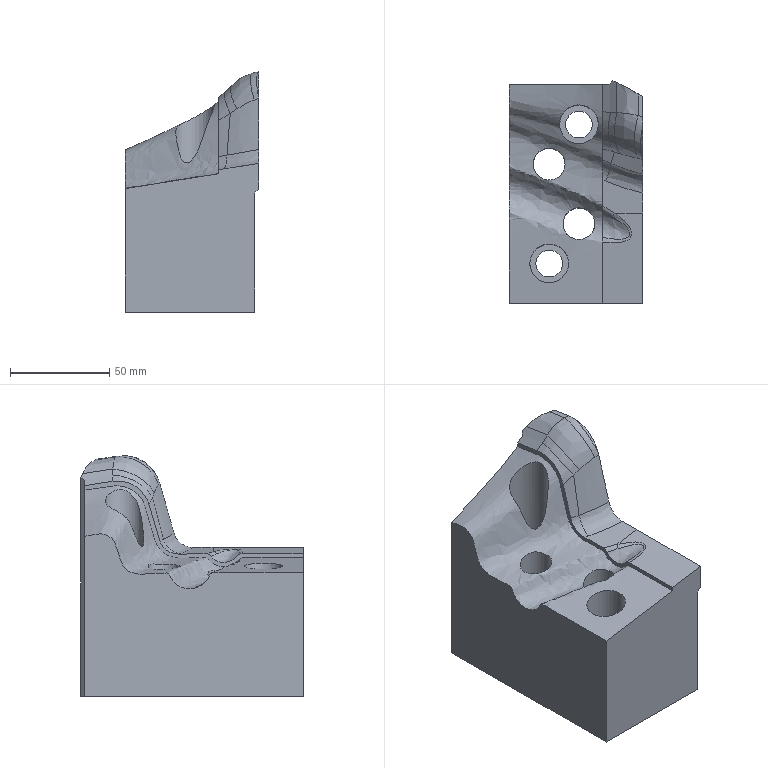Part | NX | features solid 2 | 1 solid | 36 faces | box 67.016 x 111.935 x 121.072 mm | volume 475311 mm3 | spline 21 | plane 9 | cylinder 6 | commonest cylinder face diameters 13.5 x2 16 x2 19.5 x2